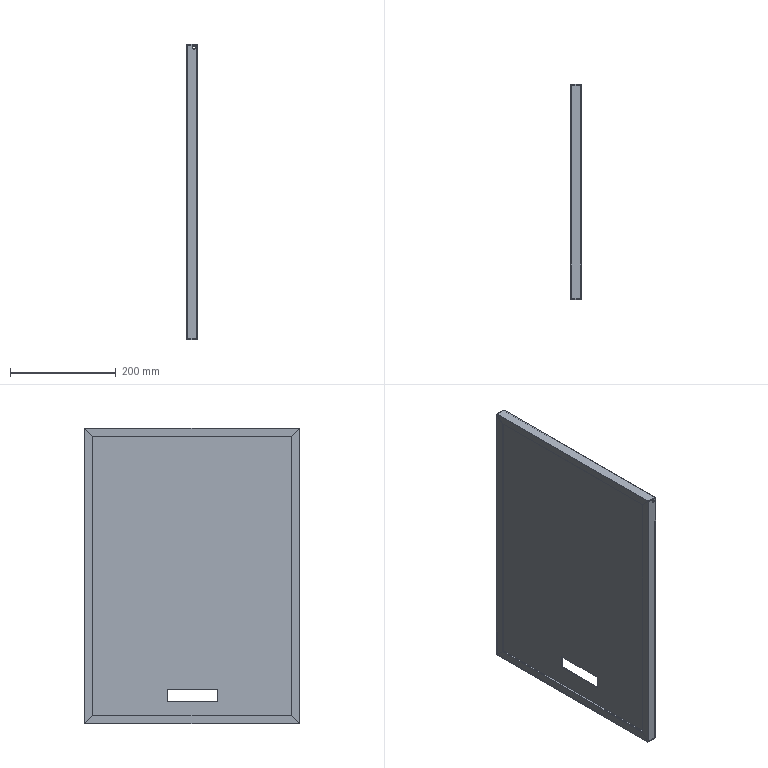Part | 1 solid | 78 faces | box 19.5 x 405 x 557 mm | volume 424280 mm3 | plane 74 | cylinder 4 | commonest cylinder face diameters 5.2 x4